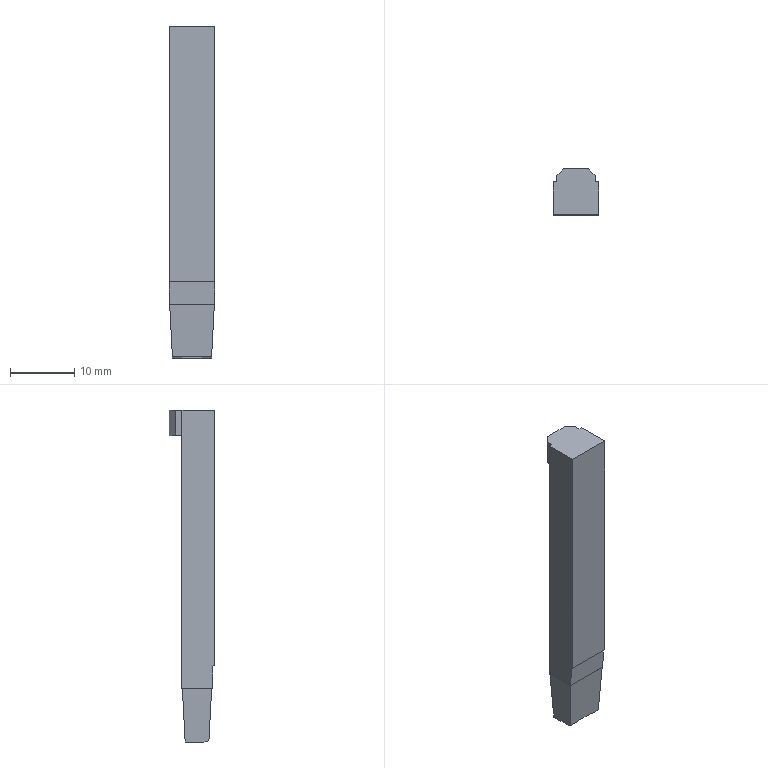Part | Creo | 1 solid | 27 faces | box 7.052 x 7.112 x 51.658 mm | volume 1819 mm3 | plane 27
STEP:
#1=CARTESIAN_POINT('',(0.,0.,0.));
#2=DIRECTION('',(0.,0.,1.));
#3=DIRECTION('',(1.,0.,0.));
#4=AXIS2_PLACEMENT_3D('',#1,#2,#3);
#5=CARTESIAN_POINT('',(-30.237,-86.843,42.593));
#6=VERTEX_POINT('',#5);
#7=CARTESIAN_POINT('',(-30.237,-82.138,42.593));
#8=VERTEX_POINT('',#7);
#9=CARTESIAN_POINT('',(-30.237,-86.843,42.593));
#10=DIRECTION('',(0.,1.,0.));
#11=VECTOR('',#10,4.704);
#12=LINE('',#9,#11);
#13=EDGE_CURVE('',#6,#8,#12,.T.);
#14=ORIENTED_EDGE('',*,*,#13,.F.);
#15=CARTESIAN_POINT('',(-23.185,-86.843,42.593));
#16=VERTEX_POINT('',#15);
#17=CARTESIAN_POINT('',(-30.237,-86.843,42.593));
#18=DIRECTION('',(1.,0.,0.));
#19=VECTOR('',#18,7.052);
#20=LINE('',#17,#19);
#21=EDGE_CURVE('',#6,#16,#20,.T.);
#22=ORIENTED_EDGE('',*,*,#21,.T.);
#23=CARTESIAN_POINT('',(-23.185,-82.138,42.593));
#24=VERTEX_POINT('',#23);
#25=CARTESIAN_POINT('',(-23.185,-82.138,42.593));
#26=DIRECTION('',(0.,-1.,0.));
#27=VECTOR('',#26,4.704);
#28=LINE('',#25,#27);
#29=EDGE_CURVE('',#24,#16,#28,.T.);
#30=ORIENTED_EDGE('',*,*,#29,.F.);
#31=CARTESIAN_POINT('',(-23.185,-82.138,42.593));
#32=DIRECTION('',(-1.,0.,0.));
#33=VECTOR('',#32,7.052);
#34=LINE('',#31,#33);
#35=EDGE_CURVE('',#24,#8,#34,.T.);
#36=ORIENTED_EDGE('',*,*,#35,.T.);
#37=EDGE_LOOP('',(#14,#22,#30,#36));
#38=FACE_OUTER_BOUND('',#37,.F.);
#39=CARTESIAN_POINT('',(-30.187,-86.751,42.593));
#40=VERTEX_POINT('',#39);
#41=CARTESIAN_POINT('',(-23.235,-86.751,42.593));
#42=VERTEX_POINT('',#41);
#43=CARTESIAN_POINT('',(-30.187,-86.751,42.593));
#44=DIRECTION('',(1.,0.,0.));
#45=VECTOR('',#44,6.952);
#46=LINE('',#43,#45);
#47=EDGE_CURVE('',#40,#42,#46,.T.);
#48=ORIENTED_EDGE('',*,*,#47,.F.);
#49=CARTESIAN_POINT('',(-30.187,-82.188,42.593));
#50=VERTEX_POINT('',#49);
#51=CARTESIAN_POINT('',(-30.187,-82.188,42.593));
#52=DIRECTION('',(0.,-1.,0.));
#53=VECTOR('',#52,4.562);
#54=LINE('',#51,#53);
#55=EDGE_CURVE('',#50,#40,#54,.T.);
#56=ORIENTED_EDGE('',*,*,#55,.F.);
#57=CARTESIAN_POINT('',(-23.235,-82.188,42.593));
#58=VERTEX_POINT('',#57);
#59=CARTESIAN_POINT('',(-23.235,-82.188,42.593));
#60=DIRECTION('',(-1.,0.,0.));
#61=VECTOR('',#60,6.952);
#62=LINE('',#59,#61);
#63=EDGE_CURVE('',#58,#50,#62,.T.);
#64=ORIENTED_EDGE('',*,*,#63,.F.);
#65=CARTESIAN_POINT('',(-23.235,-86.751,42.593));
#66=DIRECTION('',(0.,1.,0.));
#67=VECTOR('',#66,4.562);
#68=LINE('',#65,#67);
#69=EDGE_CURVE('',#42,#58,#68,.T.);
#70=ORIENTED_EDGE('',*,*,#69,.F.);
#71=EDGE_LOOP('',(#48,#56,#64,#70));
#72=FACE_BOUND('',#71,.F.);
#73=CARTESIAN_POINT('',(-0.07825,-88.35,42.593));
#74=DIRECTION('',(0.,0.,1.));
#75=DIRECTION('',(0.,-1.,0.));
#76=AXIS2_PLACEMENT_3D('',#73,#74,#75);
#77=PLANE('',#76);
#78=ADVANCED_FACE('',(#38,#72),#77,.F.);
#79=CARTESIAN_POINT('',(-30.237,-86.965,46.111));
#80=VERTEX_POINT('',#79);
#81=CARTESIAN_POINT('',(-30.237,-86.843,42.593));
#82=DIRECTION('',(0.,-0.0349,0.9994));
#83=VECTOR('',#82,3.52);
#84=LINE('',#81,#83);
#85=EDGE_CURVE('',#6,#80,#84,.T.);
#86=ORIENTED_EDGE('',*,*,#85,.F.);
#87=ORIENTED_EDGE('',*,*,#13,.T.);
#88=CARTESIAN_POINT('',(-30.237,-82.138,85.91));
#89=VERTEX_POINT('',#88);
#90=CARTESIAN_POINT('',(-30.237,-82.138,85.91));
#91=DIRECTION('',(0.,0.,-1.));
#92=VECTOR('',#91,43.316);
#93=LINE('',#90,#92);
#94=EDGE_CURVE('',#89,#8,#93,.T.);
#95=ORIENTED_EDGE('',*,*,#94,.F.);
#96=CARTESIAN_POINT('',(-30.237,-87.251,85.91));
#97=VERTEX_POINT('',#96);
#98=CARTESIAN_POINT('',(-30.237,-82.138,85.91));
#99=DIRECTION('',(0.,-1.,0.));
#100=VECTOR('',#99,5.112);
#101=LINE('',#98,#100);
#102=EDGE_CURVE('',#89,#97,#101,.T.);
#103=ORIENTED_EDGE('',*,*,#102,.T.);
#104=CARTESIAN_POINT('',(-30.237,-87.251,46.111));
#105=VERTEX_POINT('',#104);
#106=CARTESIAN_POINT('',(-30.237,-87.251,85.91));
#107=DIRECTION('',(0.,0.,-1.));
#108=VECTOR('',#107,39.799);
#109=LINE('',#106,#108);
#110=EDGE_CURVE('',#97,#105,#109,.T.);
#111=ORIENTED_EDGE('',*,*,#110,.T.);
#112=CARTESIAN_POINT('',(-30.237,-87.251,46.111));
#113=DIRECTION('',(0.,1.,0.));
#114=VECTOR('',#113,0.2855);
#115=LINE('',#112,#114);
#116=EDGE_CURVE('',#105,#80,#115,.T.);
#117=ORIENTED_EDGE('',*,*,#116,.T.);
#118=EDGE_LOOP('',(#86,#87,#95,#103,#111,#117));
#119=FACE_OUTER_BOUND('',#118,.F.);
#120=CARTESIAN_POINT('',(-30.237,-84.72,21.593));
#121=DIRECTION('',(-1.,0.,0.));
#122=DIRECTION('',(0.,0.,1.));
#123=AXIS2_PLACEMENT_3D('',#120,#121,#122);
#124=PLANE('',#123);
#125=ADVANCED_FACE('',(#119),#124,.T.);
#126=CARTESIAN_POINT('',(-23.185,-86.965,46.111));
#127=VERTEX_POINT('',#126);
#128=CARTESIAN_POINT('',(-30.237,-86.965,46.111));
#129=DIRECTION('',(1.,0.,0.));
#130=VECTOR('',#129,7.052);
#131=LINE('',#128,#130);
#132=EDGE_CURVE('',#80,#127,#131,.T.);
#133=ORIENTED_EDGE('',*,*,#132,.T.);
#134=CARTESIAN_POINT('',(-23.185,-86.965,46.111));
#135=DIRECTION('',(0.,0.0349,-0.9994));
#136=VECTOR('',#135,3.52);
#137=LINE('',#134,#136);
#138=EDGE_CURVE('',#127,#16,#137,.T.);
#139=ORIENTED_EDGE('',*,*,#138,.T.);
#140=ORIENTED_EDGE('',*,*,#21,.F.);
#141=ORIENTED_EDGE('',*,*,#85,.T.);
#142=EDGE_LOOP('',(#133,#139,#140,#141));
#143=FACE_OUTER_BOUND('',#142,.F.);
#144=CARTESIAN_POINT('',(-43.293,-86.843,42.593));
#145=DIRECTION('',(0.,-0.9994,-0.0349));
#146=DIRECTION('',(0.,0.0349,-0.9994));
#147=AXIS2_PLACEMENT_3D('',#144,#145,#146);
#148=PLANE('',#147);
#149=ADVANCED_FACE('',(#143),#148,.T.);
#150=ORIENTED_EDGE('',*,*,#116,.F.);
#151=CARTESIAN_POINT('',(-23.185,-87.251,46.111));
#152=VERTEX_POINT('',#151);
#153=CARTESIAN_POINT('',(-23.185,-87.251,46.111));
#154=DIRECTION('',(-1.,0.,0.));
#155=VECTOR('',#154,7.052);
#156=LINE('',#153,#155);
#157=EDGE_CURVE('',#152,#105,#156,.T.);
#158=ORIENTED_EDGE('',*,*,#157,.F.);
#159=CARTESIAN_POINT('',(-23.185,-86.965,46.111));
#160=DIRECTION('',(0.,-1.,0.));
#161=VECTOR('',#160,0.2855);
#162=LINE('',#159,#161);
#163=EDGE_CURVE('',#127,#152,#162,.T.);
#164=ORIENTED_EDGE('',*,*,#163,.F.);
#165=ORIENTED_EDGE('',*,*,#132,.F.);
#166=EDGE_LOOP('',(#150,#158,#164,#165));
#167=FACE_OUTER_BOUND('',#166,.F.);
#168=CARTESIAN_POINT('',(-45.303,-88.35,46.111));
#169=DIRECTION('',(0.,0.,1.));
#170=DIRECTION('',(-1.,0.,0.));
#171=AXIS2_PLACEMENT_3D('',#168,#169,#170);
#172=PLANE('',#171);
#173=ADVANCED_FACE('',(#167),#172,.F.);
#174=ORIENTED_EDGE('',*,*,#110,.F.);
#175=CARTESIAN_POINT('',(-23.185,-87.251,85.91));
#176=VERTEX_POINT('',#175);
#177=CARTESIAN_POINT('',(-30.237,-87.251,85.91));
#178=DIRECTION('',(1.,0.,0.));
#179=VECTOR('',#178,7.052);
#180=LINE('',#177,#179);
#181=EDGE_CURVE('',#97,#176,#180,.T.);
#182=ORIENTED_EDGE('',*,*,#181,.T.);
#183=CARTESIAN_POINT('',(-23.185,-87.251,85.91));
#184=DIRECTION('',(0.,0.,-1.));
#185=VECTOR('',#184,39.799);
#186=LINE('',#183,#185);
#187=EDGE_CURVE('',#176,#152,#186,.T.);
#188=ORIENTED_EDGE('',*,*,#187,.T.);
#189=ORIENTED_EDGE('',*,*,#157,.T.);
#190=EDGE_LOOP('',(#174,#182,#188,#189));
#191=FACE_OUTER_BOUND('',#190,.F.);
#192=CARTESIAN_POINT('',(-26.711,-87.251,21.593));
#193=DIRECTION('',(0.,-1.,0.));
#194=DIRECTION('',(0.,0.,-1.));
#195=AXIS2_PLACEMENT_3D('',#192,#193,#194);
#196=PLANE('',#195);
#197=ADVANCED_FACE('',(#191),#196,.T.);
#198=CARTESIAN_POINT('',(-23.735,-82.138,85.91));
#199=VERTEX_POINT('',#198);
#200=CARTESIAN_POINT('',(-23.735,-81.138,85.91));
#201=VERTEX_POINT('',#200);
#202=CARTESIAN_POINT('',(-23.735,-82.138,85.91));
#203=DIRECTION('',(0.,1.,0.));
#204=VECTOR('',#203,1.);
#205=LINE('',#202,#204);
#206=EDGE_CURVE('',#199,#201,#205,.T.);
#207=ORIENTED_EDGE('',*,*,#206,.F.);
#208=CARTESIAN_POINT('',(-23.185,-82.138,85.91));
#209=VERTEX_POINT('',#208);
#210=CARTESIAN_POINT('',(-23.185,-82.138,85.91));
#211=DIRECTION('',(-1.,0.,0.));
#212=VECTOR('',#211,0.55);
#213=LINE('',#210,#212);
#214=EDGE_CURVE('',#209,#199,#213,.T.);
#215=ORIENTED_EDGE('',*,*,#214,.F.);
#216=CARTESIAN_POINT('',(-23.185,-87.251,85.91));
#217=DIRECTION('',(0.,1.,0.));
#218=VECTOR('',#217,5.112);
#219=LINE('',#216,#218);
#220=EDGE_CURVE('',#176,#209,#219,.T.);
#221=ORIENTED_EDGE('',*,*,#220,.F.);
#222=ORIENTED_EDGE('',*,*,#181,.F.);
#223=ORIENTED_EDGE('',*,*,#102,.F.);
#224=CARTESIAN_POINT('',(-29.687,-82.138,85.91));
#225=VERTEX_POINT('',#224);
#226=CARTESIAN_POINT('',(-29.687,-82.138,85.91));
#227=DIRECTION('',(-1.,0.,0.));
#228=VECTOR('',#227,0.55);
#229=LINE('',#226,#228);
#230=EDGE_CURVE('',#225,#89,#229,.T.);
#231=ORIENTED_EDGE('',*,*,#230,.F.);
#232=CARTESIAN_POINT('',(-29.687,-81.138,85.91));
#233=VERTEX_POINT('',#232);
#234=CARTESIAN_POINT('',(-29.687,-81.138,85.91));
#235=DIRECTION('',(0.,-1.,0.));
#236=VECTOR('',#235,1.);
#237=LINE('',#234,#236);
#238=EDGE_CURVE('',#233,#225,#237,.T.);
#239=ORIENTED_EDGE('',*,*,#238,.F.);
#240=CARTESIAN_POINT('',(-28.687,-80.138,85.91));
#241=VERTEX_POINT('',#240);
#242=CARTESIAN_POINT('',(-28.687,-80.138,85.91));
#243=DIRECTION('',(-0.7071,-0.7071,0.));
#244=VECTOR('',#243,1.414);
#245=LINE('',#242,#244);
#246=EDGE_CURVE('',#241,#233,#245,.T.);
#247=ORIENTED_EDGE('',*,*,#246,.F.);
#248=CARTESIAN_POINT('',(-24.735,-80.138,85.91));
#249=VERTEX_POINT('',#248);
#250=CARTESIAN_POINT('',(-24.735,-80.138,85.91));
#251=DIRECTION('',(-1.,0.,0.));
#252=VECTOR('',#251,3.952);
#253=LINE('',#250,#252);
#254=EDGE_CURVE('',#249,#241,#253,.T.);
#255=ORIENTED_EDGE('',*,*,#254,.F.);
#256=CARTESIAN_POINT('',(-23.735,-81.138,85.91));
#257=DIRECTION('',(-0.7071,0.7071,0.));
#258=VECTOR('',#257,1.414);
#259=LINE('',#256,#258);
#260=EDGE_CURVE('',#201,#249,#259,.T.);
#261=ORIENTED_EDGE('',*,*,#260,.F.);
#262=EDGE_LOOP('',(#207,#215,#221,#222,#223,#231,#239,#247,#255,#261));
#263=FACE_OUTER_BOUND('',#262,.F.);
#264=CARTESIAN_POINT('',(62.144,-0.4125,85.91));
#265=DIRECTION('',(0.,0.,1.));
#266=DIRECTION('',(0.,1.,0.));
#267=AXIS2_PLACEMENT_3D('',#264,#265,#266);
#268=PLANE('',#267);
#269=ADVANCED_FACE('',(#263),#268,.T.);
#270=CARTESIAN_POINT('',(-23.735,-81.138,81.91));
#271=VERTEX_POINT('',#270);
#272=CARTESIAN_POINT('',(-23.735,-82.138,81.91));
#273=VERTEX_POINT('',#272);
#274=CARTESIAN_POINT('',(-23.735,-81.138,81.91));
#275=DIRECTION('',(0.,-1.,0.));
#276=VECTOR('',#275,1.);
#277=LINE('',#274,#276);
#278=EDGE_CURVE('',#271,#273,#277,.T.);
#279=ORIENTED_EDGE('',*,*,#278,.T.);
#280=CARTESIAN_POINT('',(-23.735,-82.138,81.91));
#281=DIRECTION('',(0.,0.,1.));
#282=VECTOR('',#281,4.);
#283=LINE('',#280,#282);
#284=EDGE_CURVE('',#273,#199,#283,.T.);
#285=ORIENTED_EDGE('',*,*,#284,.T.);
#286=ORIENTED_EDGE('',*,*,#206,.T.);
#287=CARTESIAN_POINT('',(-23.735,-81.138,85.91));
#288=DIRECTION('',(0.,0.,-1.));
#289=VECTOR('',#288,4.);
#290=LINE('',#287,#289);
#291=EDGE_CURVE('',#201,#271,#290,.T.);
#292=ORIENTED_EDGE('',*,*,#291,.T.);
#293=EDGE_LOOP('',(#279,#285,#286,#292));
#294=FACE_OUTER_BOUND('',#293,.F.);
#295=CARTESIAN_POINT('',(-23.735,-81.688,81.91));
#296=DIRECTION('',(1.,0.,0.));
#297=DIRECTION('',(0.,0.,-1.));
#298=AXIS2_PLACEMENT_3D('',#295,#296,#297);
#299=PLANE('',#298);
#300=ADVANCED_FACE('',(#294),#299,.T.);
#301=CARTESIAN_POINT('',(-28.687,-80.138,81.91));
#302=VERTEX_POINT('',#301);
#303=CARTESIAN_POINT('',(-24.735,-80.138,81.91));
#304=VERTEX_POINT('',#303);
#305=CARTESIAN_POINT('',(-28.687,-80.138,81.91));
#306=DIRECTION('',(1.,0.,0.));
#307=VECTOR('',#306,3.952);
#308=LINE('',#305,#307);
#309=EDGE_CURVE('',#302,#304,#308,.T.);
#310=ORIENTED_EDGE('',*,*,#309,.F.);
#311=CARTESIAN_POINT('',(-29.687,-81.138,81.91));
#312=VERTEX_POINT('',#311);
#313=CARTESIAN_POINT('',(-29.687,-81.138,81.91));
#314=DIRECTION('',(0.7071,0.7071,0.));
#315=VECTOR('',#314,1.414);
#316=LINE('',#313,#315);
#317=EDGE_CURVE('',#312,#302,#316,.T.);
#318=ORIENTED_EDGE('',*,*,#317,.F.);
#319=CARTESIAN_POINT('',(-29.687,-82.138,81.91));
#320=VERTEX_POINT('',#319);
#321=CARTESIAN_POINT('',(-29.687,-82.138,81.91));
#322=DIRECTION('',(0.,1.,0.));
#323=VECTOR('',#322,1.);
#324=LINE('',#321,#323);
#325=EDGE_CURVE('',#320,#312,#324,.T.);
#326=ORIENTED_EDGE('',*,*,#325,.F.);
#327=CARTESIAN_POINT('',(-29.687,-82.138,81.91));
#328=DIRECTION('',(1.,0.,0.));
#329=VECTOR('',#328,5.952);
#330=LINE('',#327,#329);
#331=EDGE_CURVE('',#320,#273,#330,.T.);
#332=ORIENTED_EDGE('',*,*,#331,.T.);
#333=ORIENTED_EDGE('',*,*,#278,.F.);
#334=CARTESIAN_POINT('',(-24.735,-80.138,81.91));
#335=DIRECTION('',(0.7071,-0.7071,0.));
#336=VECTOR('',#335,1.414);
#337=LINE('',#334,#336);
#338=EDGE_CURVE('',#304,#271,#337,.T.);
#339=ORIENTED_EDGE('',*,*,#338,.F.);
#340=EDGE_LOOP('',(#310,#318,#326,#332,#333,#339));
#341=FACE_OUTER_BOUND('',#340,.F.);
#342=CARTESIAN_POINT('',(-26.711,-81.688,81.91));
#343=DIRECTION('',(0.,0.,-1.));
#344=DIRECTION('',(-1.,0.,0.));
#345=AXIS2_PLACEMENT_3D('',#342,#343,#344);
#346=PLANE('',#345);
#347=ADVANCED_FACE('',(#341),#346,.T.);
#348=ORIENTED_EDGE('',*,*,#254,.T.);
#349=CARTESIAN_POINT('',(-28.687,-80.138,85.91));
#350=DIRECTION('',(0.,0.,-1.));
#351=VECTOR('',#350,4.);
#352=LINE('',#349,#351);
#353=EDGE_CURVE('',#241,#302,#352,.T.);
#354=ORIENTED_EDGE('',*,*,#353,.T.);
#355=ORIENTED_EDGE('',*,*,#309,.T.);
#356=CARTESIAN_POINT('',(-24.735,-80.138,81.91));
#357=DIRECTION('',(0.,0.,1.));
#358=VECTOR('',#357,4.);
#359=LINE('',#356,#358);
#360=EDGE_CURVE('',#304,#249,#359,.T.);
#361=ORIENTED_EDGE('',*,*,#360,.T.);
#362=EDGE_LOOP('',(#348,#354,#355,#361));
#363=FACE_OUTER_BOUND('',#362,.F.);
#364=CARTESIAN_POINT('',(-26.711,-80.138,81.91));
#365=DIRECTION('',(0.,1.,0.));
#366=DIRECTION('',(0.,0.,1.));
#367=AXIS2_PLACEMENT_3D('',#364,#365,#366);
#368=PLANE('',#367);
#369=ADVANCED_FACE('',(#363),#368,.T.);
#370=ORIENTED_EDGE('',*,*,#317,.T.);
#371=ORIENTED_EDGE('',*,*,#353,.F.);
#372=ORIENTED_EDGE('',*,*,#246,.T.);
#373=CARTESIAN_POINT('',(-29.687,-81.138,81.91));
#374=DIRECTION('',(0.,0.,1.));
#375=VECTOR('',#374,4.);
#376=LINE('',#373,#375);
#377=EDGE_CURVE('',#312,#233,#376,.T.);
#378=ORIENTED_EDGE('',*,*,#377,.F.);
#379=EDGE_LOOP('',(#370,#371,#372,#378));
#380=FACE_OUTER_BOUND('',#379,.F.);
#381=CARTESIAN_POINT('',(-28.687,-80.138,81.91));
#382=DIRECTION('',(0.7071,-0.7071,0.));
#383=DIRECTION('',(0.,0.,1.));
#384=AXIS2_PLACEMENT_3D('',#381,#382,#383);
#385=PLANE('',#384);
#386=ADVANCED_FACE('',(#380),#385,.F.);
#387=ORIENTED_EDGE('',*,*,#238,.T.);
#388=CARTESIAN_POINT('',(-29.687,-82.138,85.91));
#389=DIRECTION('',(0.,0.,-1.));
#390=VECTOR('',#389,4.);
#391=LINE('',#388,#390);
#392=EDGE_CURVE('',#225,#320,#391,.T.);
#393=ORIENTED_EDGE('',*,*,#392,.T.);
#394=ORIENTED_EDGE('',*,*,#325,.T.);
#395=ORIENTED_EDGE('',*,*,#377,.T.);
#396=EDGE_LOOP('',(#387,#393,#394,#395));
#397=FACE_OUTER_BOUND('',#396,.F.);
#398=CARTESIAN_POINT('',(-29.687,-81.688,81.91));
#399=DIRECTION('',(-1.,0.,0.));
#400=DIRECTION('',(0.,0.,1.));
#401=AXIS2_PLACEMENT_3D('',#398,#399,#400);
#402=PLANE('',#401);
#403=ADVANCED_FACE('',(#397),#402,.T.);
#404=ORIENTED_EDGE('',*,*,#35,.F.);
#405=CARTESIAN_POINT('',(-23.185,-82.138,85.91));
#406=DIRECTION('',(0.,0.,-1.));
#407=VECTOR('',#406,43.316);
#408=LINE('',#405,#407);
#409=EDGE_CURVE('',#209,#24,#408,.T.);
#410=ORIENTED_EDGE('',*,*,#409,.F.);
#411=ORIENTED_EDGE('',*,*,#214,.T.);
#412=ORIENTED_EDGE('',*,*,#284,.F.);
#413=ORIENTED_EDGE('',*,*,#331,.F.);
#414=ORIENTED_EDGE('',*,*,#392,.F.);
#415=ORIENTED_EDGE('',*,*,#230,.T.);
#416=ORIENTED_EDGE('',*,*,#94,.T.);
#417=EDGE_LOOP('',(#404,#410,#411,#412,#413,#414,#415,#416));
#418=FACE_OUTER_BOUND('',#417,.F.);
#419=CARTESIAN_POINT('',(-26.711,-82.138,21.593));
#420=DIRECTION('',(0.,1.,0.));
#421=DIRECTION('',(0.,0.,1.));
#422=AXIS2_PLACEMENT_3D('',#419,#420,#421);
#423=PLANE('',#422);
#424=ADVANCED_FACE('',(#418),#423,.T.);
#425=ORIENTED_EDGE('',*,*,#187,.F.);
#426=ORIENTED_EDGE('',*,*,#220,.T.);
#427=ORIENTED_EDGE('',*,*,#409,.T.);
#428=ORIENTED_EDGE('',*,*,#29,.T.);
#429=ORIENTED_EDGE('',*,*,#138,.F.);
#430=ORIENTED_EDGE('',*,*,#163,.T.);
#431=EDGE_LOOP('',(#425,#426,#427,#428,#429,#430));
#432=FACE_OUTER_BOUND('',#431,.F.);
#433=CARTESIAN_POINT('',(-23.185,-84.72,21.593));
#434=DIRECTION('',(1.,0.,0.));
#435=DIRECTION('',(0.,0.,-1.));
#436=AXIS2_PLACEMENT_3D('',#433,#434,#435);
#437=PLANE('',#436);
#438=ADVANCED_FACE('',(#432),#437,.T.);
#439=ORIENTED_EDGE('',*,*,#338,.T.);
#440=ORIENTED_EDGE('',*,*,#291,.F.);
#441=ORIENTED_EDGE('',*,*,#260,.T.);
#442=ORIENTED_EDGE('',*,*,#360,.F.);
#443=EDGE_LOOP('',(#439,#440,#441,#442));
#444=FACE_OUTER_BOUND('',#443,.F.);
#445=CARTESIAN_POINT('',(-23.735,-81.138,81.91));
#446=DIRECTION('',(-0.7071,-0.7071,0.));
#447=DIRECTION('',(0.,0.,1.));
#448=AXIS2_PLACEMENT_3D('',#445,#446,#447);
#449=PLANE('',#448);
#450=ADVANCED_FACE('',(#444),#449,.F.);
#451=ORIENTED_EDGE('',*,*,#47,.T.);
#452=CARTESIAN_POINT('',(-23.661,-86.324,34.456));
#453=VERTEX_POINT('',#452);
#454=CARTESIAN_POINT('',(-23.235,-86.751,42.593));
#455=DIRECTION('',(-0.05226,0.05226,-0.9973));
#456=VECTOR('',#455,8.159);
#457=LINE('',#454,#456);
#458=EDGE_CURVE('',#42,#453,#457,.T.);
#459=ORIENTED_EDGE('',*,*,#458,.T.);
#460=CARTESIAN_POINT('',(-25.217,-86.324,34.456));
#461=VERTEX_POINT('',#460);
#462=CARTESIAN_POINT('',(-25.217,-86.324,34.456));
#463=DIRECTION('',(1.,0.,0.));
#464=VECTOR('',#463,1.556);
#465=LINE('',#462,#464);
#466=EDGE_CURVE('',#461,#453,#465,.T.);
#467=ORIENTED_EDGE('',*,*,#466,.F.);
#468=CARTESIAN_POINT('',(-25.217,-86.328,34.516));
#469=VERTEX_POINT('',#468);
#470=CARTESIAN_POINT('',(-25.217,-86.324,34.456));
#471=DIRECTION('',(-0.001066,-0.05234,0.9986));
#472=VECTOR('',#471,0.0598);
#473=LINE('',#470,#472);
#474=EDGE_CURVE('',#461,#469,#473,.T.);
#475=ORIENTED_EDGE('',*,*,#474,.T.);
#476=CARTESIAN_POINT('',(-25.219,-86.33,34.554));
#477=VERTEX_POINT('',#476);
#478=CARTESIAN_POINT('',(-25.219,-86.33,34.554));
#479=DIRECTION('',(0.05226,0.05226,-0.9973));
#480=VECTOR('',#479,0.03844);
#481=LINE('',#478,#480);
#482=EDGE_CURVE('',#477,#469,#481,.T.);
#483=ORIENTED_EDGE('',*,*,#482,.F.);
#484=CARTESIAN_POINT('',(-28.202,-86.33,34.554));
#485=VERTEX_POINT('',#484);
#486=CARTESIAN_POINT('',(-25.219,-86.33,34.554));
#487=DIRECTION('',(-1.,0.,0.));
#488=VECTOR('',#487,2.983);
#489=LINE('',#486,#488);
#490=EDGE_CURVE('',#477,#485,#489,.T.);
#491=ORIENTED_EDGE('',*,*,#490,.T.);
#492=CARTESIAN_POINT('',(-28.204,-86.328,34.516));
#493=VERTEX_POINT('',#492);
#494=CARTESIAN_POINT('',(-28.204,-86.328,34.516));
#495=DIRECTION('',(0.05226,-0.05226,0.9973));
#496=VECTOR('',#495,0.03844);
#497=LINE('',#494,#496);
#498=EDGE_CURVE('',#493,#485,#497,.T.);
#499=ORIENTED_EDGE('',*,*,#498,.F.);
#500=CARTESIAN_POINT('',(-28.204,-86.324,34.456));
#501=VERTEX_POINT('',#500);
#502=CARTESIAN_POINT('',(-28.204,-86.328,34.516));
#503=DIRECTION('',(-0.001066,0.05234,-0.9986));
#504=VECTOR('',#503,0.0598);
#505=LINE('',#502,#504);
#506=EDGE_CURVE('',#493,#501,#505,.T.);
#507=ORIENTED_EDGE('',*,*,#506,.T.);
#508=CARTESIAN_POINT('',(-29.76,-86.324,34.456));
#509=VERTEX_POINT('',#508);
#510=CARTESIAN_POINT('',(-29.76,-86.324,34.456));
#511=DIRECTION('',(1.,0.,0.));
#512=VECTOR('',#511,1.556);
#513=LINE('',#510,#512);
#514=EDGE_CURVE('',#509,#501,#513,.T.);
#515=ORIENTED_EDGE('',*,*,#514,.F.);
#516=CARTESIAN_POINT('',(-30.187,-86.751,42.593));
#517=DIRECTION('',(0.05226,0.05226,-0.9973));
#518=VECTOR('',#517,8.159);
#519=LINE('',#516,#518);
#520=EDGE_CURVE('',#40,#509,#519,.T.);
#521=ORIENTED_EDGE('',*,*,#520,.F.);
#522=EDGE_LOOP('',(#451,#459,#467,#475,#483,#491,#499,#507,#515,#521));
#523=FACE_OUTER_BOUND('',#522,.F.);
#524=CARTESIAN_POINT('',(-32.335,-86.34,34.755));
#525=DIRECTION('',(0.,0.9986,0.05234));
#526=DIRECTION('',(1.,0.,0.));
#527=AXIS2_PLACEMENT_3D('',#524,#525,#526);
#528=PLANE('',#527);
#529=ADVANCED_FACE('',(#523),#528,.F.);
#530=ORIENTED_EDGE('',*,*,#69,.T.);
#531=CARTESIAN_POINT('',(-23.672,-82.625,34.252));
#532=VERTEX_POINT('',#531);
#533=CARTESIAN_POINT('',(-23.235,-82.188,42.593));
#534=DIRECTION('',(-0.05226,-0.05226,-0.9973));
#535=VECTOR('',#534,8.364);
#536=LINE('',#533,#535);
#537=EDGE_CURVE('',#58,#532,#536,.T.);
#538=ORIENTED_EDGE('',*,*,#537,.T.);
#539=CARTESIAN_POINT('',(-23.672,-85.561,34.252));
#540=VERTEX_POINT('',#539);
#541=CARTESIAN_POINT('',(-23.672,-82.625,34.252));
#542=DIRECTION('',(0.,-1.,0.));
#543=VECTOR('',#542,2.936);
#544=LINE('',#541,#543);
#545=EDGE_CURVE('',#532,#540,#544,.T.);
#546=ORIENTED_EDGE('',*,*,#545,.T.);
#547=CARTESIAN_POINT('',(-23.661,-86.324,34.456));
#548=DIRECTION('',(-0.01356,0.9658,-0.2588));
#549=VECTOR('',#548,0.79);
#550=LINE('',#547,#549);
#551=EDGE_CURVE('',#453,#540,#550,.T.);
#552=ORIENTED_EDGE('',*,*,#551,.F.);
#553=ORIENTED_EDGE('',*,*,#458,.F.);
#554=EDGE_LOOP('',(#530,#538,#546,#552,#553));
#555=FACE_OUTER_BOUND('',#554,.F.);
#556=CARTESIAN_POINT('',(-23.646,-82.188,34.752));
#557=DIRECTION('',(0.9986,0.,-0.05234));
#558=DIRECTION('',(0.,-1.,0.));
#559=AXIS2_PLACEMENT_3D('',#556,#557,#558);
#560=PLANE('',#559);
#561=ADVANCED_FACE('',(#555),#560,.T.);
#562=ORIENTED_EDGE('',*,*,#63,.T.);
#563=CARTESIAN_POINT('',(-29.75,-82.625,34.252));
#564=VERTEX_POINT('',#563);
#565=CARTESIAN_POINT('',(-30.187,-82.188,42.593));
#566=DIRECTION('',(0.05226,-0.05226,-0.9973));
#567=VECTOR('',#566,8.364);
#568=LINE('',#565,#567);
#569=EDGE_CURVE('',#50,#564,#568,.T.);
#570=ORIENTED_EDGE('',*,*,#569,.T.);
#571=CARTESIAN_POINT('',(-29.75,-82.625,34.252));
#572=DIRECTION('',(1.,0.,0.));
#573=VECTOR('',#572,6.078);
#574=LINE('',#571,#573);
#575=EDGE_CURVE('',#564,#532,#574,.T.);
#576=ORIENTED_EDGE('',*,*,#575,.T.);
#577=ORIENTED_EDGE('',*,*,#537,.F.);
#578=EDGE_LOOP('',(#562,#570,#576,#577));
#579=FACE_OUTER_BOUND('',#578,.F.);
#580=CARTESIAN_POINT('',(-20.081,-82.32,40.081));
#581=DIRECTION('',(0.,0.9986,-0.05234));
#582=DIRECTION('',(-1.,0.,0.));
#583=AXIS2_PLACEMENT_3D('',#580,#581,#582);
#584=PLANE('',#583);
#585=ADVANCED_FACE('',(#579),#584,.T.);
#586=ORIENTED_EDGE('',*,*,#55,.T.);
#587=ORIENTED_EDGE('',*,*,#520,.T.);
#588=CARTESIAN_POINT('',(-29.75,-85.561,34.252));
#589=VERTEX_POINT('',#588);
#590=CARTESIAN_POINT('',(-29.75,-85.561,34.252));
#591=DIRECTION('',(-0.01356,-0.9658,0.2588));
#592=VECTOR('',#591,0.79);
#593=LINE('',#590,#592);
#594=EDGE_CURVE('',#589,#509,#593,.T.);
#595=ORIENTED_EDGE('',*,*,#594,.F.);
#596=CARTESIAN_POINT('',(-29.75,-85.561,34.252));
#597=DIRECTION('',(0.,1.,0.));
#598=VECTOR('',#597,2.936);
#599=LINE('',#596,#598);
#600=EDGE_CURVE('',#589,#564,#599,.T.);
#601=ORIENTED_EDGE('',*,*,#600,.T.);
#602=ORIENTED_EDGE('',*,*,#569,.F.);
#603=EDGE_LOOP('',(#586,#587,#595,#601,#602));
#604=FACE_OUTER_BOUND('',#603,.F.);
#605=CARTESIAN_POINT('',(-29.776,-82.188,34.752));
#606=DIRECTION('',(-0.9986,0.,-0.05234));
#607=DIRECTION('',(0.,-1.,0.));
#608=AXIS2_PLACEMENT_3D('',#605,#606,#607);
#609=PLANE('',#608);
#610=ADVANCED_FACE('',(#604),#609,.T.);
#611=ORIENTED_EDGE('',*,*,#514,.T.);
#612=CARTESIAN_POINT('',(-28.218,-85.561,34.252));
#613=VERTEX_POINT('',#612);
#614=CARTESIAN_POINT('',(-28.218,-85.561,34.252));
#615=DIRECTION('',(0.0169,-0.9658,0.2588));
#616=VECTOR('',#615,0.79);
#617=LINE('',#614,#616);
#618=EDGE_CURVE('',#613,#501,#617,.T.);
#619=ORIENTED_EDGE('',*,*,#618,.F.);
#620=CARTESIAN_POINT('',(-29.75,-85.561,34.252));
#621=DIRECTION('',(1.,0.,0.));
#622=VECTOR('',#621,1.532);
#623=LINE('',#620,#622);
#624=EDGE_CURVE('',#589,#613,#623,.T.);
#625=ORIENTED_EDGE('',*,*,#624,.F.);
#626=ORIENTED_EDGE('',*,*,#594,.T.);
#627=EDGE_LOOP('',(#611,#619,#625,#626));
#628=FACE_OUTER_BOUND('',#627,.F.);
#629=CARTESIAN_POINT('',(41.122,-86.47,34.496));
#630=DIRECTION('',(0.,0.2588,0.9659));
#631=DIRECTION('',(0.,0.9659,-0.2588));
#632=AXIS2_PLACEMENT_3D('',#629,#630,#631);
#633=PLANE('',#632);
#634=ADVANCED_FACE('',(#628),#633,.F.);
#635=ORIENTED_EDGE('',*,*,#618,.T.);
#636=ORIENTED_EDGE('',*,*,#506,.F.);
#637=CARTESIAN_POINT('',(-28.218,-85.537,34.252));
#638=VERTEX_POINT('',#637);
#639=CARTESIAN_POINT('',(-28.218,-85.537,34.252));
#640=DIRECTION('',(0.0166,-0.9484,0.3168));
#641=VECTOR('',#640,0.8339);
#642=LINE('',#639,#641);
#643=EDGE_CURVE('',#638,#493,#642,.T.);
#644=ORIENTED_EDGE('',*,*,#643,.F.);
#645=CARTESIAN_POINT('',(-28.218,-85.537,34.252));
#646=DIRECTION('',(0.01745,-0.9998,0.));
#647=VECTOR('',#646,0.02471);
#648=LINE('',#645,#647);
#649=EDGE_CURVE('',#638,#613,#648,.T.);
#650=ORIENTED_EDGE('',*,*,#649,.T.);
#651=EDGE_LOOP('',(#635,#636,#644,#650));
#652=FACE_OUTER_BOUND('',#651,.F.);
#653=CARTESIAN_POINT('',(-28.218,-85.594,27.72));
#654=DIRECTION('',(0.9998,0.01745,-0.0001523));
#655=DIRECTION('',(0.0001523,0.000002658,1.));
#656=AXIS2_PLACEMENT_3D('',#653,#654,#655);
#657=PLANE('',#656);
#658=ADVANCED_FACE('',(#652),#657,.T.);
#659=CARTESIAN_POINT('',(-28.202,-83.843,34.554));
#660=VERTEX_POINT('',#659);
#661=CARTESIAN_POINT('',(-28.202,-83.843,34.554));
#662=DIRECTION('',(0.,-1.,0.));
#663=VECTOR('',#662,2.486);
#664=LINE('',#661,#663);
#665=EDGE_CURVE('',#660,#485,#664,.T.);
#666=ORIENTED_EDGE('',*,*,#665,.F.);
#667=CARTESIAN_POINT('',(-28.218,-83.828,34.252));
#668=VERTEX_POINT('',#667);
#669=CARTESIAN_POINT('',(-28.202,-83.843,34.554));
#670=DIRECTION('',(-0.05226,0.05226,-0.9973));
#671=VECTOR('',#670,0.3033);
#672=LINE('',#669,#671);
#673=EDGE_CURVE('',#660,#668,#672,.T.);
#674=ORIENTED_EDGE('',*,*,#673,.T.);
#675=CARTESIAN_POINT('',(-28.218,-85.537,34.252));
#676=DIRECTION('',(0.,1.,0.));
#677=VECTOR('',#676,1.709);
#678=LINE('',#675,#677);
#679=EDGE_CURVE('',#638,#668,#678,.T.);
#680=ORIENTED_EDGE('',*,*,#679,.F.);
#681=ORIENTED_EDGE('',*,*,#643,.T.);
#682=ORIENTED_EDGE('',*,*,#498,.T.);
#683=EDGE_LOOP('',(#666,#674,#680,#681,#682));
#684=FACE_OUTER_BOUND('',#683,.F.);
#685=CARTESIAN_POINT('',(-28.218,-83.828,34.252));
#686=DIRECTION('',(0.9986,0.,-0.05234));
#687=DIRECTION('',(-0.05234,0.,-0.9986));
#688=AXIS2_PLACEMENT_3D('',#685,#686,#687);
#689=PLANE('',#688);
#690=ADVANCED_FACE('',(#684),#689,.T.);
#691=CARTESIAN_POINT('',(-25.219,-83.843,34.554));
#692=VERTEX_POINT('',#691);
#693=CARTESIAN_POINT('',(-25.219,-86.33,34.554));
#694=DIRECTION('',(0.,1.,0.));
#695=VECTOR('',#694,2.486);
#696=LINE('',#693,#695);
#697=EDGE_CURVE('',#477,#692,#696,.T.);
#698=ORIENTED_EDGE('',*,*,#697,.T.);
#699=CARTESIAN_POINT('',(-25.219,-83.843,34.554));
#700=DIRECTION('',(-1.,0.,0.));
#701=VECTOR('',#700,2.983);
#702=LINE('',#699,#701);
#703=EDGE_CURVE('',#692,#660,#702,.T.);
#704=ORIENTED_EDGE('',*,*,#703,.T.);
#705=ORIENTED_EDGE('',*,*,#665,.T.);
#706=ORIENTED_EDGE('',*,*,#490,.F.);
#707=EDGE_LOOP('',(#698,#704,#705,#706));
#708=FACE_OUTER_BOUND('',#707,.F.);
#709=CARTESIAN_POINT('',(25.047,-88.35,34.554));
#710=DIRECTION('',(0.,0.,-1.));
#711=DIRECTION('',(-1.,0.,0.));
#712=AXIS2_PLACEMENT_3D('',#709,#710,#711);
#713=PLANE('',#712);
#714=ADVANCED_FACE('',(#708),#713,.T.);
#715=CARTESIAN_POINT('',(-25.203,-85.537,34.252));
#716=VERTEX_POINT('',#715);
#717=CARTESIAN_POINT('',(-25.217,-86.328,34.516));
#718=DIRECTION('',(0.0166,0.9484,-0.3168));
#719=VECTOR('',#718,0.8339);
#720=LINE('',#717,#719);
#721=EDGE_CURVE('',#469,#716,#720,.T.);
#722=ORIENTED_EDGE('',*,*,#721,.T.);
#723=CARTESIAN_POINT('',(-25.203,-83.828,34.252));
#724=VERTEX_POINT('',#723);
#725=CARTESIAN_POINT('',(-25.203,-83.828,34.252));
#726=DIRECTION('',(0.,-1.,0.));
#727=VECTOR('',#726,1.709);
#728=LINE('',#725,#727);
#729=EDGE_CURVE('',#724,#716,#728,.T.);
#730=ORIENTED_EDGE('',*,*,#729,.F.);
#731=CARTESIAN_POINT('',(-25.219,-83.843,34.554));
#732=DIRECTION('',(0.05226,0.05226,-0.9973));
#733=VECTOR('',#732,0.3033);
#734=LINE('',#731,#733);
#735=EDGE_CURVE('',#692,#724,#734,.T.);
#736=ORIENTED_EDGE('',*,*,#735,.F.);
#737=ORIENTED_EDGE('',*,*,#697,.F.);
#738=ORIENTED_EDGE('',*,*,#482,.T.);
#739=EDGE_LOOP('',(#722,#730,#736,#737,#738));
#740=FACE_OUTER_BOUND('',#739,.F.);
#741=CARTESIAN_POINT('',(-25.203,-83.828,34.252));
#742=DIRECTION('',(-0.9986,0.,-0.05234));
#743=DIRECTION('',(-0.05234,0.,0.9986));
#744=AXIS2_PLACEMENT_3D('',#741,#742,#743);
#745=PLANE('',#744);
#746=ADVANCED_FACE('',(#740),#745,.T.);
#747=ORIENTED_EDGE('',*,*,#474,.F.);
#748=CARTESIAN_POINT('',(-25.204,-85.561,34.252));
#749=VERTEX_POINT('',#748);
#750=CARTESIAN_POINT('',(-25.217,-86.324,34.456));
#751=DIRECTION('',(0.0169,0.9658,-0.2588));
#752=VECTOR('',#751,0.79);
#753=LINE('',#750,#752);
#754=EDGE_CURVE('',#461,#749,#753,.T.);
#755=ORIENTED_EDGE('',*,*,#754,.T.);
#756=CARTESIAN_POINT('',(-25.204,-85.561,34.252));
#757=DIRECTION('',(0.01745,0.9998,0.));
#758=VECTOR('',#757,0.02471);
#759=LINE('',#756,#758);
#760=EDGE_CURVE('',#749,#716,#759,.T.);
#761=ORIENTED_EDGE('',*,*,#760,.T.);
#762=ORIENTED_EDGE('',*,*,#721,.F.);
#763=EDGE_LOOP('',(#747,#755,#761,#762));
#764=FACE_OUTER_BOUND('',#763,.F.);
#765=CARTESIAN_POINT('',(-25.203,-85.519,36.262));
#766=DIRECTION('',(-0.9998,0.01745,-0.0001523));
#767=DIRECTION('',(0.0001523,-0.000002658,-1.));
#768=AXIS2_PLACEMENT_3D('',#765,#766,#767);
#769=PLANE('',#768);
#770=ADVANCED_FACE('',(#764),#769,.T.);
#771=ORIENTED_EDGE('',*,*,#754,.F.);
#772=ORIENTED_EDGE('',*,*,#466,.T.);
#773=ORIENTED_EDGE('',*,*,#551,.T.);
#774=CARTESIAN_POINT('',(-25.204,-85.561,34.252));
#775=DIRECTION('',(1.,0.,0.));
#776=VECTOR('',#775,1.532);
#777=LINE('',#774,#776);
#778=EDGE_CURVE('',#749,#540,#777,.T.);
#779=ORIENTED_EDGE('',*,*,#778,.F.);
#780=EDGE_LOOP('',(#771,#772,#773,#779));
#781=FACE_OUTER_BOUND('',#780,.F.);
#782=CARTESIAN_POINT('',(41.122,-86.47,34.496));
#783=DIRECTION('',(0.,0.2588,0.9659));
#784=DIRECTION('',(0.,0.9659,-0.2588));
#785=AXIS2_PLACEMENT_3D('',#782,#783,#784);
#786=PLANE('',#785);
#787=ADVANCED_FACE('',(#781),#786,.F.);
#788=ORIENTED_EDGE('',*,*,#600,.F.);
#789=ORIENTED_EDGE('',*,*,#624,.T.);
#790=ORIENTED_EDGE('',*,*,#649,.F.);
#791=ORIENTED_EDGE('',*,*,#679,.T.);
#792=CARTESIAN_POINT('',(-25.203,-83.828,34.252));
#793=DIRECTION('',(-1.,0.,0.));
#794=VECTOR('',#793,3.015);
#795=LINE('',#792,#794);
#796=EDGE_CURVE('',#724,#668,#795,.T.);
#797=ORIENTED_EDGE('',*,*,#796,.F.);
#798=ORIENTED_EDGE('',*,*,#729,.T.);
#799=ORIENTED_EDGE('',*,*,#760,.F.);
#800=ORIENTED_EDGE('',*,*,#778,.T.);
#801=ORIENTED_EDGE('',*,*,#545,.F.);
#802=ORIENTED_EDGE('',*,*,#575,.F.);
#803=EDGE_LOOP('',(#788,#789,#790,#791,#797,#798,#799,#800,#801,#802));
#804=FACE_OUTER_BOUND('',#803,.F.);
#805=CARTESIAN_POINT('',(-28.218,-83.828,34.252));
#806=DIRECTION('',(0.,0.,1.));
#807=DIRECTION('',(0.,1.,0.));
#808=AXIS2_PLACEMENT_3D('',#805,#806,#807);
#809=PLANE('',#808);
#810=ADVANCED_FACE('',(#804),#809,.F.);
#811=ORIENTED_EDGE('',*,*,#673,.F.);
#812=ORIENTED_EDGE('',*,*,#703,.F.);
#813=ORIENTED_EDGE('',*,*,#735,.T.);
#814=ORIENTED_EDGE('',*,*,#796,.T.);
#815=EDGE_LOOP('',(#811,#812,#813,#814));
#816=FACE_OUTER_BOUND('',#815,.F.);
#817=CARTESIAN_POINT('',(-28.218,-83.828,34.252));
#818=DIRECTION('',(0.,-0.9986,-0.05234));
#819=DIRECTION('',(0.,-0.05234,0.9986));
#820=AXIS2_PLACEMENT_3D('',#817,#818,#819);
#821=PLANE('',#820);
#822=ADVANCED_FACE('',(#816),#821,.T.);
#823=CLOSED_SHELL('',(#78,#125,#149,#173,#197,#269,#300,#347,#369,#386,#403,#424,#438,#450,#529,#561,#585,#610,#634,#658,#690,#714,#746,#770,#787,#810,#822));
#824=MANIFOLD_SOLID_BREP('',#823);
#825=(LENGTH_UNIT()NAMED_UNIT(*)SI_UNIT(.MILLI.,.METRE.));
#826=UNCERTAINTY_MEASURE_WITH_UNIT(LENGTH_MEASURE(0.005262),#825,'','');
#827=(NAMED_UNIT(*)PLANE_ANGLE_UNIT()SI_UNIT($,.RADIAN.));
#828=PLANE_ANGLE_MEASURE_WITH_UNIT(PLANE_ANGLE_MEASURE(0.01745),#827);
#829=(CONVERSION_BASED_UNIT('DEGREE',#828)NAMED_UNIT(*)PLANE_ANGLE_UNIT());
#830=(NAMED_UNIT(*)SI_UNIT($,.STERADIAN.)SOLID_ANGLE_UNIT());
#831=(GEOMETRIC_REPRESENTATION_CONTEXT(3)GLOBAL_UNCERTAINTY_ASSIGNED_CONTEXT((#826))GLOBAL_UNIT_ASSIGNED_CONTEXT((#825,#829,#830))REPRESENTATION_CONTEXT('',''));
#832=ADVANCED_BREP_SHAPE_REPRESENTATION('',(#4,#824),#831);